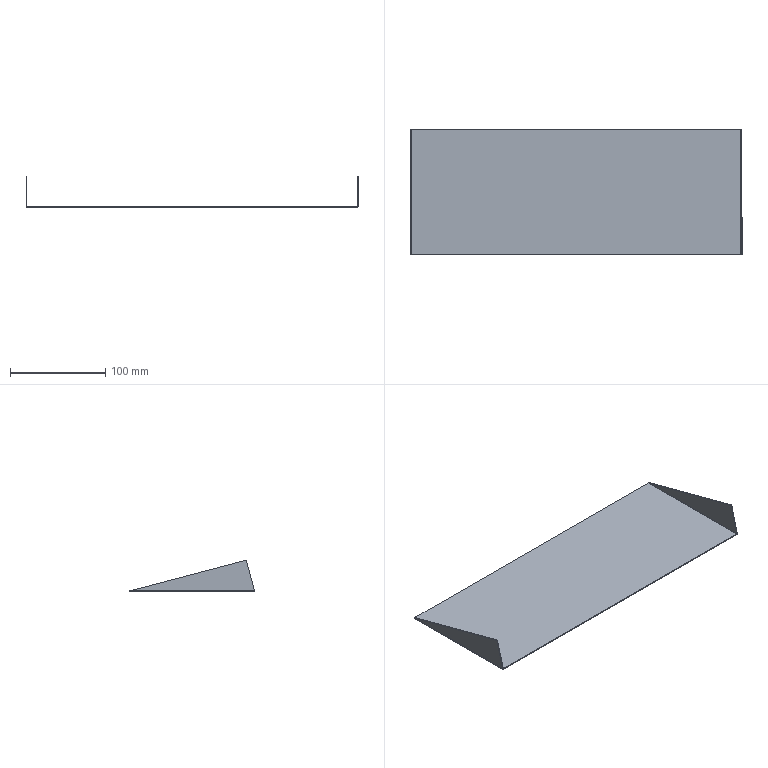Part | SolidWorks | features EdgeFlange 1, FlatPattern 1, MirrorPattern 1, SMBaseFlange 1, SheetMetal 1 | 1 solid | 20 faces | box 349.001 x 131.5 x 33.5 mm | volume 50088 mm3 | plane 12 | spline 4 | cylinder 4 | commonest cylinder face diameters 0.4 x2 2.4 x2
STEP:
#1=CARTESIAN_POINT('',(173.3,65.75,-1.));
#2=VERTEX_POINT('',#1);
#3=CARTESIAN_POINT('',(173.3,-65.75,-1.));
#4=VERTEX_POINT('',#3);
#5=CARTESIAN_POINT('',(173.3,65.75,-1.));
#6=DIRECTION('',(0.,-1.,0.));
#7=VECTOR('',#6,1000.);
#8=LINE('',#5,#7);
#9=EDGE_CURVE('',#2,#4,#8,.T.);
#10=ORIENTED_EDGE('',*,*,#9,.T.);
#11=CARTESIAN_POINT('',(-173.3,-65.75,-1.));
#12=VERTEX_POINT('',#11);
#13=CARTESIAN_POINT('',(-174.5,-65.75,-1.));
#14=DIRECTION('',(1.,0.,0.));
#15=VECTOR('',#14,1000.);
#16=LINE('',#13,#15);
#17=EDGE_CURVE('',#12,#4,#16,.T.);
#18=ORIENTED_EDGE('',*,*,#17,.F.);
#19=CARTESIAN_POINT('',(-173.3,65.75,-1.));
#20=VERTEX_POINT('',#19);
#21=CARTESIAN_POINT('',(-173.3,-65.75,-1.));
#22=DIRECTION('',(0.,1.,0.));
#23=VECTOR('',#22,1000.);
#24=LINE('',#21,#23);
#25=EDGE_CURVE('',#12,#20,#24,.T.);
#26=ORIENTED_EDGE('',*,*,#25,.T.);
#27=CARTESIAN_POINT('',(-174.5,65.75,-1.));
#28=DIRECTION('',(-1.,0.,0.));
#29=VECTOR('',#28,1000.);
#30=LINE('',#27,#29);
#31=EDGE_CURVE('',#2,#20,#30,.T.);
#32=ORIENTED_EDGE('',*,*,#31,.F.);
#33=EDGE_LOOP('',(#10,#18,#26,#32));
#34=FACE_OUTER_BOUND('',#33,.T.);
#35=CARTESIAN_POINT('',(0.,0.,-1.));
#36=DIRECTION('',(0.,0.,1.));
#37=DIRECTION('',(1.,0.,0.));
#38=AXIS2_PLACEMENT_3D('',#35,#36,#37);
#39=PLANE('',#38);
#40=ADVANCED_FACE('',(#34),#39,.F.);
#41=CARTESIAN_POINT('',(-173.3,-65.75,0.));
#42=VERTEX_POINT('',#41);
#43=CARTESIAN_POINT('',(173.3,-65.75,0.));
#44=VERTEX_POINT('',#43);
#45=CARTESIAN_POINT('',(-174.5,-65.75,0.));
#46=DIRECTION('',(1.,0.,0.));
#47=VECTOR('',#46,1000.);
#48=LINE('',#45,#47);
#49=EDGE_CURVE('',#42,#44,#48,.T.);
#50=ORIENTED_EDGE('',*,*,#49,.T.);
#51=CARTESIAN_POINT('',(173.3,65.75,0.));
#52=VERTEX_POINT('',#51);
#53=CARTESIAN_POINT('',(173.3,65.75,0.));
#54=DIRECTION('',(0.,-1.,0.));
#55=VECTOR('',#54,1000.);
#56=LINE('',#53,#55);
#57=EDGE_CURVE('',#52,#44,#56,.T.);
#58=ORIENTED_EDGE('',*,*,#57,.F.);
#59=CARTESIAN_POINT('',(-173.3,65.75,0.));
#60=VERTEX_POINT('',#59);
#61=CARTESIAN_POINT('',(-174.5,65.75,0.));
#62=DIRECTION('',(-1.,0.,0.));
#63=VECTOR('',#62,1000.);
#64=LINE('',#61,#63);
#65=EDGE_CURVE('',#52,#60,#64,.T.);
#66=ORIENTED_EDGE('',*,*,#65,.T.);
#67=CARTESIAN_POINT('',(-173.3,-65.75,0.));
#68=DIRECTION('',(0.,1.,0.));
#69=VECTOR('',#68,1000.);
#70=LINE('',#67,#69);
#71=EDGE_CURVE('',#42,#60,#70,.T.);
#72=ORIENTED_EDGE('',*,*,#71,.F.);
#73=EDGE_LOOP('',(#50,#58,#66,#72));
#74=FACE_OUTER_BOUND('',#73,.T.);
#75=CARTESIAN_POINT('',(0.,0.,0.));
#76=DIRECTION('',(0.,0.,1.));
#77=DIRECTION('',(1.,0.,0.));
#78=AXIS2_PLACEMENT_3D('',#75,#76,#77);
#79=PLANE('',#78);
#80=ADVANCED_FACE('',(#74),#79,.T.);
#81=ORIENTED_EDGE('',*,*,#65,.F.);
#82=CARTESIAN_POINT('',(173.3,65.75,0.));
#83=DIRECTION('',(0.,0.,-1.));
#84=VECTOR('',#83,1000.);
#85=LINE('',#82,#84);
#86=EDGE_CURVE('',#52,#2,#85,.T.);
#87=ORIENTED_EDGE('',*,*,#86,.T.);
#88=ORIENTED_EDGE('',*,*,#31,.T.);
#89=CARTESIAN_POINT('',(-173.3,65.75,0.));
#90=DIRECTION('',(0.,0.,-1.));
#91=VECTOR('',#90,1000.);
#92=LINE('',#89,#91);
#93=EDGE_CURVE('',#60,#20,#92,.T.);
#94=ORIENTED_EDGE('',*,*,#93,.F.);
#95=EDGE_LOOP('',(#81,#87,#88,#94));
#96=FACE_OUTER_BOUND('',#95,.T.);
#97=CARTESIAN_POINT('',(-174.5,65.75,-1.));
#98=DIRECTION('',(0.,1.,0.));
#99=DIRECTION('',(0.,0.,1.));
#100=AXIS2_PLACEMENT_3D('',#97,#98,#99);
#101=PLANE('',#100);
#102=ADVANCED_FACE('',(#96),#101,.T.);
#103=CARTESIAN_POINT('',(173.3,-65.75,0.));
#104=DIRECTION('',(0.,0.,-1.));
#105=VECTOR('',#104,1000.);
#106=LINE('',#103,#105);
#107=EDGE_CURVE('',#44,#4,#106,.T.);
#108=ORIENTED_EDGE('',*,*,#107,.F.);
#109=ORIENTED_EDGE('',*,*,#49,.F.);
#110=CARTESIAN_POINT('',(-173.3,-65.75,0.));
#111=DIRECTION('',(0.,0.,-1.));
#112=VECTOR('',#111,1000.);
#113=LINE('',#110,#112);
#114=EDGE_CURVE('',#42,#12,#113,.T.);
#115=ORIENTED_EDGE('',*,*,#114,.T.);
#116=ORIENTED_EDGE('',*,*,#17,.T.);
#117=EDGE_LOOP('',(#108,#109,#115,#116));
#118=FACE_OUTER_BOUND('',#117,.T.);
#119=CARTESIAN_POINT('',(-174.5,-65.75,-1.));
#120=DIRECTION('',(0.,-1.,0.));
#121=DIRECTION('',(0.,0.,-1.));
#122=AXIS2_PLACEMENT_3D('',#119,#120,#121);
#123=PLANE('',#122);
#124=ADVANCED_FACE('',(#118),#123,.T.);
#125=CARTESIAN_POINT('',(-173.5,64.994,0.2));
#126=VERTEX_POINT('',#125);
#127=CARTESIAN_POINT('',(-174.5,64.994,0.2));
#128=VERTEX_POINT('',#127);
#129=CARTESIAN_POINT('',(-174.5,64.994,0.2));
#130=DIRECTION('',(-1.,0.,0.));
#131=VECTOR('',#130,1000.);
#132=LINE('',#129,#131);
#133=EDGE_CURVE('',#126,#128,#132,.T.);
#134=ORIENTED_EDGE('',*,*,#133,.F.);
#135=CARTESIAN_POINT('',(-173.3,65.75,0.));
#136=CARTESIAN_POINT('',(-173.352,65.624,0.));
#137=CARTESIAN_POINT('',(-173.404,65.498,0.02155));
#138=CARTESIAN_POINT('',(-173.478,65.246,0.0956));
#139=CARTESIAN_POINT('',(-173.5,65.12,0.1476));
#140=CARTESIAN_POINT('',(-173.5,64.994,0.2));
#141=B_SPLINE_CURVE_WITH_KNOTS('',3,(#135,#136,#137,#138,#139,#140),.UNSPECIFIED.,.F.,.F.,(4,2,4),(0.,0.5,1.),.UNSPECIFIED.);
#142=EDGE_CURVE('',#60,#126,#141,.T.);
#143=ORIENTED_EDGE('',*,*,#142,.F.);
#144=ORIENTED_EDGE('',*,*,#93,.T.);
#145=CARTESIAN_POINT('',(-173.3,65.75,-1.));
#146=CARTESIAN_POINT('',(-173.459,65.686,-1.));
#147=CARTESIAN_POINT('',(-173.612,65.625,-0.9695));
#148=CARTESIAN_POINT('',(-173.905,65.498,-0.8485));
#149=CARTESIAN_POINT('',(-174.036,65.436,-0.7607));
#150=CARTESIAN_POINT('',(-174.26,65.309,-0.5373));
#151=CARTESIAN_POINT('',(-174.348,65.246,-0.4052));
#152=CARTESIAN_POINT('',(-174.469,65.12,-0.1142));
#153=CARTESIAN_POINT('',(-174.5,65.057,0.04141));
#154=CARTESIAN_POINT('',(-174.5,64.994,0.2));
#155=B_SPLINE_CURVE_WITH_KNOTS('',3,(#145,#146,#147,#148,#149,#150,#151,#152,#153,#154),.UNSPECIFIED.,.F.,.F.,(4,2,2,2,4),(0.,0.0005039,0.001008,0.001512,0.002016),.UNSPECIFIED.);
#156=EDGE_CURVE('',#20,#128,#155,.T.);
#157=ORIENTED_EDGE('',*,*,#156,.T.);
#158=EDGE_LOOP('',(#134,#143,#144,#157));
#159=FACE_OUTER_BOUND('',#158,.T.);
#160=CARTESIAN_POINT('',(-173.3,65.75,-1.01));
#161=CARTESIAN_POINT('',(-173.458,65.687,-1.01));
#162=CARTESIAN_POINT('',(-173.617,65.624,-0.9785));
#163=CARTESIAN_POINT('',(-173.909,65.498,-0.8573));
#164=CARTESIAN_POINT('',(-174.044,65.435,-0.7676));
#165=CARTESIAN_POINT('',(-174.268,65.309,-0.5436));
#166=CARTESIAN_POINT('',(-174.357,65.246,-0.4094));
#167=CARTESIAN_POINT('',(-174.479,65.12,-0.1167));
#168=CARTESIAN_POINT('',(-174.51,65.057,0.04159));
#169=CARTESIAN_POINT('',(-174.51,64.994,0.2));
#170=CARTESIAN_POINT('',(-173.3,65.75,-1.));
#171=CARTESIAN_POINT('',(-173.457,65.687,-1.));
#172=CARTESIAN_POINT('',(-173.614,65.624,-0.9688));
#173=CARTESIAN_POINT('',(-173.904,65.498,-0.8485));
#174=CARTESIAN_POINT('',(-174.037,65.435,-0.7596));
#175=CARTESIAN_POINT('',(-174.26,65.309,-0.5375));
#176=CARTESIAN_POINT('',(-174.349,65.246,-0.4043));
#177=CARTESIAN_POINT('',(-174.469,65.12,-0.1141));
#178=CARTESIAN_POINT('',(-174.5,65.057,0.0429));
#179=CARTESIAN_POINT('',(-174.5,64.994,0.2));
#180=CARTESIAN_POINT('',(-173.3,65.75,0.));
#181=CARTESIAN_POINT('',(-173.326,65.687,0.));
#182=CARTESIAN_POINT('',(-173.352,65.624,0.005205));
#183=CARTESIAN_POINT('',(-173.401,65.498,0.02524));
#184=CARTESIAN_POINT('',(-173.423,65.435,0.04007));
#185=CARTESIAN_POINT('',(-173.46,65.309,0.07709));
#186=CARTESIAN_POINT('',(-173.475,65.246,0.09928));
#187=CARTESIAN_POINT('',(-173.495,65.12,0.1477));
#188=CARTESIAN_POINT('',(-173.5,65.057,0.1738));
#189=CARTESIAN_POINT('',(-173.5,64.994,0.2));
#190=B_SPLINE_SURFACE_WITH_KNOTS('',1,3,((#160,#161,#162,#163,#164,#165,#166,#167,#168,#169),(#170,#171,#172,#173,#174,#175,#176,#177,#178,#179),(#180,#181,#182,#183,#184,#185,#186,#187,#188,#189)),.UNSPECIFIED.,.F.,.F.,.F.,(2,1,2),(4,2,2,2,4),(-0.01,0.,1.),(0.,0.25,0.5,0.75,1.),.UNSPECIFIED.);
#191=ADVANCED_FACE('',(#159),#190,.F.);
#192=CARTESIAN_POINT('',(-173.5,-65.697,0.2));
#193=VERTEX_POINT('',#192);
#194=CARTESIAN_POINT('',(-173.5,-65.697,0.2));
#195=CARTESIAN_POINT('',(-173.5,-65.706,0.1476));
#196=CARTESIAN_POINT('',(-173.478,-65.715,0.0956));
#197=CARTESIAN_POINT('',(-173.404,-65.732,0.02155));
#198=CARTESIAN_POINT('',(-173.352,-65.741,0.));
#199=CARTESIAN_POINT('',(-173.3,-65.75,0.));
#200=B_SPLINE_CURVE_WITH_KNOTS('',3,(#194,#195,#196,#197,#198,#199),.UNSPECIFIED.,.F.,.F.,(4,2,4),(0.,0.5,1.),.UNSPECIFIED.);
#201=EDGE_CURVE('',#193,#42,#200,.T.);
#202=ORIENTED_EDGE('',*,*,#201,.F.);
#203=CARTESIAN_POINT('',(-174.5,-65.697,0.2));
#204=VERTEX_POINT('',#203);
#205=CARTESIAN_POINT('',(-173.5,-65.697,0.2));
#206=DIRECTION('',(-1.,0.,0.));
#207=VECTOR('',#206,1000.);
#208=LINE('',#205,#207);
#209=EDGE_CURVE('',#193,#204,#208,.T.);
#210=ORIENTED_EDGE('',*,*,#209,.T.);
#211=CARTESIAN_POINT('',(-174.5,-65.697,0.2));
#212=CARTESIAN_POINT('',(-174.5,-65.702,0.04292));
#213=CARTESIAN_POINT('',(-174.469,-65.706,-0.1141));
#214=CARTESIAN_POINT('',(-174.349,-65.715,-0.4043));
#215=CARTESIAN_POINT('',(-174.26,-65.719,-0.5375));
#216=CARTESIAN_POINT('',(-174.037,-65.728,-0.7596));
#217=CARTESIAN_POINT('',(-173.904,-65.732,-0.8485));
#218=CARTESIAN_POINT('',(-173.614,-65.741,-0.9688));
#219=CARTESIAN_POINT('',(-173.457,-65.746,-1.));
#220=CARTESIAN_POINT('',(-173.3,-65.75,-1.));
#221=B_SPLINE_CURVE_WITH_KNOTS('',3,(#211,#212,#213,#214,#215,#216,#217,#218,#219,#220),.UNSPECIFIED.,.F.,.F.,(4,2,2,2,4),(0.,0.25,0.5,0.75,1.),.UNSPECIFIED.);
#222=EDGE_CURVE('',#204,#12,#221,.T.);
#223=ORIENTED_EDGE('',*,*,#222,.T.);
#224=ORIENTED_EDGE('',*,*,#114,.F.);
#225=EDGE_LOOP('',(#202,#210,#223,#224));
#226=FACE_OUTER_BOUND('',#225,.T.);
#227=CARTESIAN_POINT('',(-174.51,-65.697,0.2));
#228=CARTESIAN_POINT('',(-174.51,-65.702,0.04158));
#229=CARTESIAN_POINT('',(-174.479,-65.706,-0.1167));
#230=CARTESIAN_POINT('',(-174.357,-65.715,-0.4094));
#231=CARTESIAN_POINT('',(-174.268,-65.719,-0.5436));
#232=CARTESIAN_POINT('',(-174.044,-65.728,-0.7676));
#233=CARTESIAN_POINT('',(-173.909,-65.732,-0.8573));
#234=CARTESIAN_POINT('',(-173.617,-65.741,-0.9785));
#235=CARTESIAN_POINT('',(-173.458,-65.746,-1.01));
#236=CARTESIAN_POINT('',(-173.3,-65.75,-1.01));
#237=CARTESIAN_POINT('',(-174.5,-65.697,0.2));
#238=CARTESIAN_POINT('',(-174.5,-65.702,0.04289));
#239=CARTESIAN_POINT('',(-174.469,-65.706,-0.1141));
#240=CARTESIAN_POINT('',(-174.349,-65.715,-0.4043));
#241=CARTESIAN_POINT('',(-174.26,-65.719,-0.5375));
#242=CARTESIAN_POINT('',(-174.037,-65.728,-0.7596));
#243=CARTESIAN_POINT('',(-173.904,-65.732,-0.8485));
#244=CARTESIAN_POINT('',(-173.614,-65.741,-0.9688));
#245=CARTESIAN_POINT('',(-173.457,-65.746,-1.));
#246=CARTESIAN_POINT('',(-173.3,-65.75,-1.));
#247=CARTESIAN_POINT('',(-173.5,-65.697,0.2));
#248=CARTESIAN_POINT('',(-173.5,-65.702,0.1738));
#249=CARTESIAN_POINT('',(-173.495,-65.706,0.1477));
#250=CARTESIAN_POINT('',(-173.475,-65.715,0.09928));
#251=CARTESIAN_POINT('',(-173.46,-65.719,0.07709));
#252=CARTESIAN_POINT('',(-173.423,-65.728,0.04007));
#253=CARTESIAN_POINT('',(-173.401,-65.732,0.02524));
#254=CARTESIAN_POINT('',(-173.352,-65.741,0.005205));
#255=CARTESIAN_POINT('',(-173.326,-65.746,0.));
#256=CARTESIAN_POINT('',(-173.3,-65.75,0.));
#257=CARTESIAN_POINT('',(-173.49,-65.697,0.2));
#258=CARTESIAN_POINT('',(-173.49,-65.702,0.1751));
#259=CARTESIAN_POINT('',(-173.485,-65.706,0.1503));
#260=CARTESIAN_POINT('',(-173.466,-65.715,0.1044));
#261=CARTESIAN_POINT('',(-173.452,-65.719,0.0833));
#262=CARTESIAN_POINT('',(-173.417,-65.728,0.04814));
#263=CARTESIAN_POINT('',(-173.396,-65.732,0.03407));
#264=CARTESIAN_POINT('',(-173.35,-65.741,0.01504));
#265=CARTESIAN_POINT('',(-173.325,-65.746,0.0101));
#266=CARTESIAN_POINT('',(-173.3,-65.75,0.0101));
#267=B_SPLINE_SURFACE_WITH_KNOTS('',1,3,((#227,#228,#229,#230,#231,#232,#233,#234,#235,#236),(#237,#238,#239,#240,#241,#242,#243,#244,#245,#246),(#247,#248,#249,#250,#251,#252,#253,#254,#255,#256),(#257,#258,#259,#260,#261,#262,#263,#264,#265,#266)),.UNSPECIFIED.,.F.,.F.,.F.,(2,1,1,2),(4,2,2,2,4),(-0.01,0.,1.,1.01),(0.,0.25,0.5,0.75,1.),.UNSPECIFIED.);
#268=ADVANCED_FACE('',(#226),#267,.F.);
#269=ORIENTED_EDGE('',*,*,#25,.F.);
#270=ORIENTED_EDGE('',*,*,#222,.F.);
#271=CARTESIAN_POINT('',(-174.5,64.994,0.2));
#272=DIRECTION('',(0.,1.,0.));
#273=VECTOR('',#272,1000.);
#274=LINE('',#271,#273);
#275=EDGE_CURVE('',#204,#128,#274,.T.);
#276=ORIENTED_EDGE('',*,*,#275,.T.);
#277=ORIENTED_EDGE('',*,*,#156,.F.);
#278=EDGE_LOOP('',(#269,#270,#276,#277));
#279=FACE_OUTER_BOUND('',#278,.T.);
#280=CARTESIAN_POINT('',(-173.3,-65.75,0.2));
#281=DIRECTION('',(0.,-1.,0.));
#282=DIRECTION('',(-1.,0.,0.));
#283=AXIS2_PLACEMENT_3D('',#280,#281,#282);
#284=CYLINDRICAL_SURFACE('',#283,1.2);
#285=ADVANCED_FACE('',(#279),#284,.T.);
#286=ORIENTED_EDGE('',*,*,#71,.T.);
#287=ORIENTED_EDGE('',*,*,#142,.T.);
#288=CARTESIAN_POINT('',(-173.5,64.994,0.2));
#289=DIRECTION('',(0.,-1.,0.));
#290=VECTOR('',#289,1000.);
#291=LINE('',#288,#290);
#292=EDGE_CURVE('',#126,#193,#291,.T.);
#293=ORIENTED_EDGE('',*,*,#292,.T.);
#294=ORIENTED_EDGE('',*,*,#201,.T.);
#295=EDGE_LOOP('',(#286,#287,#293,#294));
#296=FACE_OUTER_BOUND('',#295,.T.);
#297=CARTESIAN_POINT('',(-173.3,-65.75,0.2));
#298=DIRECTION('',(0.,-1.,0.));
#299=DIRECTION('',(-1.,0.,0.));
#300=AXIS2_PLACEMENT_3D('',#297,#298,#299);
#301=CYLINDRICAL_SURFACE('',#300,0.2);
#302=ADVANCED_FACE('',(#296),#301,.F.);
#303=ORIENTED_EDGE('',*,*,#133,.T.);
#304=CARTESIAN_POINT('',(-174.5,-57.156,32.5));
#305=VERTEX_POINT('',#304);
#306=CARTESIAN_POINT('',(-174.5,4.297,16.25));
#307=DIRECTION('',(0.,0.9668,-0.2556));
#308=VECTOR('',#307,1000.);
#309=LINE('',#306,#308);
#310=EDGE_CURVE('',#305,#128,#309,.T.);
#311=ORIENTED_EDGE('',*,*,#310,.F.);
#312=CARTESIAN_POINT('',(-173.5,-57.156,32.5));
#313=VERTEX_POINT('',#312);
#314=CARTESIAN_POINT('',(-174.5,-57.156,32.5));
#315=DIRECTION('',(1.,0.,0.));
#316=VECTOR('',#315,1000.);
#317=LINE('',#314,#316);
#318=EDGE_CURVE('',#305,#313,#317,.T.);
#319=ORIENTED_EDGE('',*,*,#318,.T.);
#320=CARTESIAN_POINT('',(-173.5,-57.156,32.5));
#321=DIRECTION('',(0.,0.9668,-0.2556));
#322=VECTOR('',#321,1000.);
#323=LINE('',#320,#322);
#324=EDGE_CURVE('',#313,#126,#323,.T.);
#325=ORIENTED_EDGE('',*,*,#324,.T.);
#326=EDGE_LOOP('',(#303,#311,#319,#325));
#327=FACE_OUTER_BOUND('',#326,.T.);
#328=CARTESIAN_POINT('',(-174.5,-57.156,32.5));
#329=DIRECTION('',(0.,-0.2556,-0.9668));
#330=DIRECTION('',(0.,0.9668,-0.2556));
#331=AXIS2_PLACEMENT_3D('',#328,#329,#330);
#332=PLANE('',#331);
#333=ADVANCED_FACE('',(#327),#332,.F.);
#334=ORIENTED_EDGE('',*,*,#209,.F.);
#335=CARTESIAN_POINT('',(-173.5,-65.75,0.));
#336=DIRECTION('',(0.,0.2556,0.9668));
#337=VECTOR('',#336,1000.);
#338=LINE('',#335,#337);
#339=EDGE_CURVE('',#193,#313,#338,.T.);
#340=ORIENTED_EDGE('',*,*,#339,.T.);
#341=ORIENTED_EDGE('',*,*,#318,.F.);
#342=CARTESIAN_POINT('',(-174.5,-61.453,16.25));
#343=DIRECTION('',(0.,0.2556,0.9668));
#344=VECTOR('',#343,1000.);
#345=LINE('',#342,#344);
#346=EDGE_CURVE('',#204,#305,#345,.T.);
#347=ORIENTED_EDGE('',*,*,#346,.F.);
#348=EDGE_LOOP('',(#334,#340,#341,#347));
#349=FACE_OUTER_BOUND('',#348,.T.);
#350=CARTESIAN_POINT('',(-174.5,-65.75,0.));
#351=DIRECTION('',(0.,0.9668,-0.2556));
#352=DIRECTION('',(0.,0.2556,0.9668));
#353=AXIS2_PLACEMENT_3D('',#350,#351,#352);
#354=PLANE('',#353);
#355=ADVANCED_FACE('',(#349),#354,.F.);
#356=ORIENTED_EDGE('',*,*,#275,.F.);
#357=ORIENTED_EDGE('',*,*,#346,.T.);
#358=ORIENTED_EDGE('',*,*,#310,.T.);
#359=EDGE_LOOP('',(#356,#357,#358));
#360=FACE_OUTER_BOUND('',#359,.T.);
#361=CARTESIAN_POINT('',(-174.5,0.,0.));
#362=DIRECTION('',(1.,0.,0.));
#363=DIRECTION('',(0.,0.,-1.));
#364=AXIS2_PLACEMENT_3D('',#361,#362,#363);
#365=PLANE('',#364);
#366=ADVANCED_FACE('',(#360),#365,.F.);
#367=ORIENTED_EDGE('',*,*,#339,.F.);
#368=ORIENTED_EDGE('',*,*,#292,.F.);
#369=ORIENTED_EDGE('',*,*,#324,.F.);
#370=EDGE_LOOP('',(#367,#368,#369));
#371=FACE_OUTER_BOUND('',#370,.T.);
#372=CARTESIAN_POINT('',(-173.5,0.,0.));
#373=DIRECTION('',(1.,0.,0.));
#374=DIRECTION('',(0.,0.,-1.));
#375=AXIS2_PLACEMENT_3D('',#372,#373,#374);
#376=PLANE('',#375);
#377=ADVANCED_FACE('',(#371),#376,.T.);
#378=CARTESIAN_POINT('',(173.5,-65.697,0.2));
#379=VERTEX_POINT('',#378);
#380=CARTESIAN_POINT('',(174.5,-65.697,0.2));
#381=VERTEX_POINT('',#380);
#382=CARTESIAN_POINT('',(174.5,-65.697,0.2));
#383=DIRECTION('',(1.,0.,0.));
#384=VECTOR('',#383,1000.);
#385=LINE('',#382,#384);
#386=EDGE_CURVE('',#379,#381,#385,.T.);
#387=ORIENTED_EDGE('',*,*,#386,.F.);
#388=CARTESIAN_POINT('',(173.3,-65.75,0.));
#389=CARTESIAN_POINT('',(173.352,-65.741,0.));
#390=CARTESIAN_POINT('',(173.404,-65.732,0.02155));
#391=CARTESIAN_POINT('',(173.478,-65.715,0.0956));
#392=CARTESIAN_POINT('',(173.5,-65.706,0.1476));
#393=CARTESIAN_POINT('',(173.5,-65.697,0.2));
#394=B_SPLINE_CURVE_WITH_KNOTS('',3,(#388,#389,#390,#391,#392,#393),.UNSPECIFIED.,.F.,.F.,(4,2,4),(0.,0.5,1.),.UNSPECIFIED.);
#395=EDGE_CURVE('',#44,#379,#394,.T.);
#396=ORIENTED_EDGE('',*,*,#395,.F.);
#397=ORIENTED_EDGE('',*,*,#107,.T.);
#398=CARTESIAN_POINT('',(173.3,-65.75,-1.));
#399=CARTESIAN_POINT('',(173.457,-65.746,-1.));
#400=CARTESIAN_POINT('',(173.614,-65.741,-0.9688));
#401=CARTESIAN_POINT('',(173.904,-65.732,-0.8485));
#402=CARTESIAN_POINT('',(174.037,-65.728,-0.7596));
#403=CARTESIAN_POINT('',(174.26,-65.719,-0.5375));
#404=CARTESIAN_POINT('',(174.349,-65.715,-0.4043));
#405=CARTESIAN_POINT('',(174.469,-65.706,-0.1141));
#406=CARTESIAN_POINT('',(174.5,-65.702,0.04292));
#407=CARTESIAN_POINT('',(174.5,-65.697,0.2));
#408=B_SPLINE_CURVE_WITH_KNOTS('',3,(#398,#399,#400,#401,#402,#403,#404,#405,#406,#407),.UNSPECIFIED.,.F.,.F.,(4,2,2,2,4),(0.,0.25,0.5,0.75,1.),.UNSPECIFIED.);
#409=EDGE_CURVE('',#4,#381,#408,.T.);
#410=ORIENTED_EDGE('',*,*,#409,.T.);
#411=EDGE_LOOP('',(#387,#396,#397,#410));
#412=FACE_OUTER_BOUND('',#411,.T.);
#413=CARTESIAN_POINT('',(173.3,-65.75,-1.01));
#414=CARTESIAN_POINT('',(173.458,-65.746,-1.01));
#415=CARTESIAN_POINT('',(173.617,-65.741,-0.9785));
#416=CARTESIAN_POINT('',(173.909,-65.732,-0.8573));
#417=CARTESIAN_POINT('',(174.044,-65.728,-0.7676));
#418=CARTESIAN_POINT('',(174.268,-65.719,-0.5436));
#419=CARTESIAN_POINT('',(174.357,-65.715,-0.4094));
#420=CARTESIAN_POINT('',(174.479,-65.706,-0.1167));
#421=CARTESIAN_POINT('',(174.51,-65.702,0.04158));
#422=CARTESIAN_POINT('',(174.51,-65.697,0.2));
#423=CARTESIAN_POINT('',(173.3,-65.75,-1.));
#424=CARTESIAN_POINT('',(173.457,-65.746,-1.));
#425=CARTESIAN_POINT('',(173.614,-65.741,-0.9688));
#426=CARTESIAN_POINT('',(173.904,-65.732,-0.8485));
#427=CARTESIAN_POINT('',(174.037,-65.728,-0.7596));
#428=CARTESIAN_POINT('',(174.26,-65.719,-0.5375));
#429=CARTESIAN_POINT('',(174.349,-65.715,-0.4043));
#430=CARTESIAN_POINT('',(174.469,-65.706,-0.1141));
#431=CARTESIAN_POINT('',(174.5,-65.702,0.04289));
#432=CARTESIAN_POINT('',(174.5,-65.697,0.2));
#433=CARTESIAN_POINT('',(173.3,-65.75,0.));
#434=CARTESIAN_POINT('',(173.326,-65.746,0.));
#435=CARTESIAN_POINT('',(173.352,-65.741,0.005205));
#436=CARTESIAN_POINT('',(173.401,-65.732,0.02524));
#437=CARTESIAN_POINT('',(173.423,-65.728,0.04007));
#438=CARTESIAN_POINT('',(173.46,-65.719,0.07709));
#439=CARTESIAN_POINT('',(173.475,-65.715,0.09928));
#440=CARTESIAN_POINT('',(173.495,-65.706,0.1477));
#441=CARTESIAN_POINT('',(173.5,-65.702,0.1738));
#442=CARTESIAN_POINT('',(173.5,-65.697,0.2));
#443=CARTESIAN_POINT('',(173.3,-65.75,0.0101));
#444=CARTESIAN_POINT('',(173.325,-65.746,0.0101));
#445=CARTESIAN_POINT('',(173.35,-65.741,0.01504));
#446=CARTESIAN_POINT('',(173.396,-65.732,0.03407));
#447=CARTESIAN_POINT('',(173.417,-65.728,0.04814));
#448=CARTESIAN_POINT('',(173.452,-65.719,0.0833));
#449=CARTESIAN_POINT('',(173.466,-65.715,0.1044));
#450=CARTESIAN_POINT('',(173.485,-65.706,0.1503));
#451=CARTESIAN_POINT('',(173.49,-65.702,0.1751));
#452=CARTESIAN_POINT('',(173.49,-65.697,0.2));
#453=B_SPLINE_SURFACE_WITH_KNOTS('',1,3,((#413,#414,#415,#416,#417,#418,#419,#420,#421,#422),(#423,#424,#425,#426,#427,#428,#429,#430,#431,#432),(#433,#434,#435,#436,#437,#438,#439,#440,#441,#442),(#443,#444,#445,#446,#447,#448,#449,#450,#451,#452)),.UNSPECIFIED.,.F.,.F.,.F.,(2,1,1,2),(4,2,2,2,4),(-0.01,0.,1.,1.01),(0.,0.25,0.5,0.75,1.),.UNSPECIFIED.);
#454=ADVANCED_FACE('',(#412),#453,.F.);
#455=CARTESIAN_POINT('',(173.5,64.994,0.2));
#456=VERTEX_POINT('',#455);
#457=CARTESIAN_POINT('',(173.5,64.994,0.2));
#458=CARTESIAN_POINT('',(173.5,65.12,0.1476));
#459=CARTESIAN_POINT('',(173.478,65.246,0.0956));
#460=CARTESIAN_POINT('',(173.404,65.498,0.02155));
#461=CARTESIAN_POINT('',(173.352,65.624,0.));
#462=CARTESIAN_POINT('',(173.3,65.75,0.));
#463=B_SPLINE_CURVE_WITH_KNOTS('',3,(#457,#458,#459,#460,#461,#462),.UNSPECIFIED.,.F.,.F.,(4,2,4),(0.,0.5,1.),.UNSPECIFIED.);
#464=EDGE_CURVE('',#456,#52,#463,.T.);
#465=ORIENTED_EDGE('',*,*,#464,.F.);
#466=CARTESIAN_POINT('',(174.5,64.994,0.2));
#467=VERTEX_POINT('',#466);
#468=CARTESIAN_POINT('',(173.5,64.994,0.2));
#469=DIRECTION('',(1.,0.,0.));
#470=VECTOR('',#469,1000.);
#471=LINE('',#468,#470);
#472=EDGE_CURVE('',#456,#467,#471,.T.);
#473=ORIENTED_EDGE('',*,*,#472,.T.);
#474=CARTESIAN_POINT('',(174.5,64.994,0.2));
#475=CARTESIAN_POINT('',(174.5,65.057,0.04141));
#476=CARTESIAN_POINT('',(174.47,65.119,-0.1119));
#477=CARTESIAN_POINT('',(174.349,65.246,-0.4047));
#478=CARTESIAN_POINT('',(174.261,65.308,-0.5362));
#479=CARTESIAN_POINT('',(174.037,65.435,-0.7599));
#480=CARTESIAN_POINT('',(173.905,65.498,-0.8481));
#481=CARTESIAN_POINT('',(173.614,65.624,-0.9688));
#482=CARTESIAN_POINT('',(173.459,65.686,-1.));
#483=CARTESIAN_POINT('',(173.3,65.75,-1.));
#484=B_SPLINE_CURVE_WITH_KNOTS('',3,(#474,#475,#476,#477,#478,#479,#480,#481,#482,#483),.UNSPECIFIED.,.F.,.F.,(4,2,2,2,4),(0.,0.0005039,0.001008,0.001512,0.002016),.UNSPECIFIED.);
#485=EDGE_CURVE('',#467,#2,#484,.T.);
#486=ORIENTED_EDGE('',*,*,#485,.T.);
#487=ORIENTED_EDGE('',*,*,#86,.F.);
#488=EDGE_LOOP('',(#465,#473,#486,#487));
#489=FACE_OUTER_BOUND('',#488,.T.);
#490=CARTESIAN_POINT('',(174.51,64.994,0.2));
#491=CARTESIAN_POINT('',(174.51,65.057,0.04159));
#492=CARTESIAN_POINT('',(174.479,65.12,-0.1167));
#493=CARTESIAN_POINT('',(174.357,65.246,-0.4094));
#494=CARTESIAN_POINT('',(174.268,65.309,-0.5436));
#495=CARTESIAN_POINT('',(174.044,65.435,-0.7676));
#496=CARTESIAN_POINT('',(173.909,65.498,-0.8573));
#497=CARTESIAN_POINT('',(173.617,65.624,-0.9785));
#498=CARTESIAN_POINT('',(173.458,65.687,-1.01));
#499=CARTESIAN_POINT('',(173.3,65.75,-1.01));
#500=CARTESIAN_POINT('',(174.5,64.994,0.2));
#501=CARTESIAN_POINT('',(174.5,65.057,0.0429));
#502=CARTESIAN_POINT('',(174.469,65.12,-0.1141));
#503=CARTESIAN_POINT('',(174.349,65.246,-0.4043));
#504=CARTESIAN_POINT('',(174.26,65.309,-0.5375));
#505=CARTESIAN_POINT('',(174.037,65.435,-0.7596));
#506=CARTESIAN_POINT('',(173.904,65.498,-0.8485));
#507=CARTESIAN_POINT('',(173.614,65.624,-0.9688));
#508=CARTESIAN_POINT('',(173.457,65.687,-1.));
#509=CARTESIAN_POINT('',(173.3,65.75,-1.));
#510=CARTESIAN_POINT('',(173.5,64.994,0.2));
#511=CARTESIAN_POINT('',(173.5,65.057,0.1738));
#512=CARTESIAN_POINT('',(173.495,65.12,0.1477));
#513=CARTESIAN_POINT('',(173.475,65.246,0.09928));
#514=CARTESIAN_POINT('',(173.46,65.309,0.07709));
#515=CARTESIAN_POINT('',(173.423,65.435,0.04007));
#516=CARTESIAN_POINT('',(173.401,65.498,0.02524));
#517=CARTESIAN_POINT('',(173.352,65.624,0.005205));
#518=CARTESIAN_POINT('',(173.326,65.687,0.));
#519=CARTESIAN_POINT('',(173.3,65.75,0.));
#520=B_SPLINE_SURFACE_WITH_KNOTS('',1,3,((#490,#491,#492,#493,#494,#495,#496,#497,#498,#499),(#500,#501,#502,#503,#504,#505,#506,#507,#508,#509),(#510,#511,#512,#513,#514,#515,#516,#517,#518,#519)),.UNSPECIFIED.,.F.,.F.,.F.,(2,1,2),(4,2,2,2,4),(-0.01,0.,1.),(0.,0.25,0.5,0.75,1.),.UNSPECIFIED.);
#521=ADVANCED_FACE('',(#489),#520,.F.);
#522=ORIENTED_EDGE('',*,*,#9,.F.);
#523=ORIENTED_EDGE('',*,*,#485,.F.);
#524=CARTESIAN_POINT('',(174.5,-65.697,0.2));
#525=DIRECTION('',(0.,-1.,0.));
#526=VECTOR('',#525,1000.);
#527=LINE('',#524,#526);
#528=EDGE_CURVE('',#467,#381,#527,.T.);
#529=ORIENTED_EDGE('',*,*,#528,.T.);
#530=ORIENTED_EDGE('',*,*,#409,.F.);
#531=EDGE_LOOP('',(#522,#523,#529,#530));
#532=FACE_OUTER_BOUND('',#531,.T.);
#533=CARTESIAN_POINT('',(173.3,65.75,0.2));
#534=DIRECTION('',(0.,1.,0.));
#535=DIRECTION('',(1.,0.,0.));
#536=AXIS2_PLACEMENT_3D('',#533,#534,#535);
#537=CYLINDRICAL_SURFACE('',#536,1.2);
#538=ADVANCED_FACE('',(#532),#537,.T.);
#539=ORIENTED_EDGE('',*,*,#57,.T.);
#540=ORIENTED_EDGE('',*,*,#395,.T.);
#541=CARTESIAN_POINT('',(173.5,-65.697,0.2));
#542=DIRECTION('',(0.,1.,0.));
#543=VECTOR('',#542,1000.);
#544=LINE('',#541,#543);
#545=EDGE_CURVE('',#379,#456,#544,.T.);
#546=ORIENTED_EDGE('',*,*,#545,.T.);
#547=ORIENTED_EDGE('',*,*,#464,.T.);
#548=EDGE_LOOP('',(#539,#540,#546,#547));
#549=FACE_OUTER_BOUND('',#548,.T.);
#550=CARTESIAN_POINT('',(173.3,65.75,0.2));
#551=DIRECTION('',(0.,1.,0.));
#552=DIRECTION('',(1.,0.,0.));
#553=AXIS2_PLACEMENT_3D('',#550,#551,#552);
#554=CYLINDRICAL_SURFACE('',#553,0.2);
#555=ADVANCED_FACE('',(#549),#554,.F.);
#556=CARTESIAN_POINT('',(174.5,-57.156,32.5));
#557=VERTEX_POINT('',#556);
#558=CARTESIAN_POINT('',(174.5,-57.156,32.5));
#559=DIRECTION('',(0.,0.9668,-0.2556));
#560=VECTOR('',#559,1000.);
#561=LINE('',#558,#560);
#562=EDGE_CURVE('',#557,#467,#561,.T.);
#563=ORIENTED_EDGE('',*,*,#562,.T.);
#564=ORIENTED_EDGE('',*,*,#472,.F.);
#565=CARTESIAN_POINT('',(173.5,-57.156,32.5));
#566=VERTEX_POINT('',#565);
#567=CARTESIAN_POINT('',(173.5,4.297,16.25));
#568=DIRECTION('',(0.,0.9668,-0.2556));
#569=VECTOR('',#568,1000.);
#570=LINE('',#567,#569);
#571=EDGE_CURVE('',#566,#456,#570,.T.);
#572=ORIENTED_EDGE('',*,*,#571,.F.);
#573=CARTESIAN_POINT('',(174.5,-57.156,32.5));
#574=DIRECTION('',(-1.,0.,0.));
#575=VECTOR('',#574,1000.);
#576=LINE('',#573,#575);
#577=EDGE_CURVE('',#557,#566,#576,.T.);
#578=ORIENTED_EDGE('',*,*,#577,.F.);
#579=EDGE_LOOP('',(#563,#564,#572,#578));
#580=FACE_OUTER_BOUND('',#579,.T.);
#581=CARTESIAN_POINT('',(174.5,-57.156,32.5));
#582=DIRECTION('',(0.,0.2556,0.9668));
#583=DIRECTION('',(0.,-0.9668,0.2556));
#584=AXIS2_PLACEMENT_3D('',#581,#582,#583);
#585=PLANE('',#584);
#586=ADVANCED_FACE('',(#580),#585,.T.);
#587=CARTESIAN_POINT('',(173.5,-61.453,16.25));
#588=DIRECTION('',(0.,0.2556,0.9668));
#589=VECTOR('',#588,1000.);
#590=LINE('',#587,#589);
#591=EDGE_CURVE('',#379,#566,#590,.T.);
#592=ORIENTED_EDGE('',*,*,#591,.F.);
#593=ORIENTED_EDGE('',*,*,#386,.T.);
#594=CARTESIAN_POINT('',(174.5,-65.75,0.));
#595=DIRECTION('',(0.,0.2556,0.9668));
#596=VECTOR('',#595,1000.);
#597=LINE('',#594,#596);
#598=EDGE_CURVE('',#381,#557,#597,.T.);
#599=ORIENTED_EDGE('',*,*,#598,.T.);
#600=ORIENTED_EDGE('',*,*,#577,.T.);
#601=EDGE_LOOP('',(#592,#593,#599,#600));
#602=FACE_OUTER_BOUND('',#601,.T.);
#603=CARTESIAN_POINT('',(174.5,-65.75,0.));
#604=DIRECTION('',(0.,-0.9668,0.2556));
#605=DIRECTION('',(0.,-0.2556,-0.9668));
#606=AXIS2_PLACEMENT_3D('',#603,#604,#605);
#607=PLANE('',#606);
#608=ADVANCED_FACE('',(#602),#607,.T.);
#609=ORIENTED_EDGE('',*,*,#528,.F.);
#610=ORIENTED_EDGE('',*,*,#562,.F.);
#611=ORIENTED_EDGE('',*,*,#598,.F.);
#612=EDGE_LOOP('',(#609,#610,#611));
#613=FACE_OUTER_BOUND('',#612,.T.);
#614=CARTESIAN_POINT('',(174.5,0.,0.));
#615=DIRECTION('',(-1.,0.,0.));
#616=DIRECTION('',(0.,0.,-1.));
#617=AXIS2_PLACEMENT_3D('',#614,#615,#616);
#618=PLANE('',#617);
#619=ADVANCED_FACE('',(#613),#618,.F.);
#620=ORIENTED_EDGE('',*,*,#571,.T.);
#621=ORIENTED_EDGE('',*,*,#545,.F.);
#622=ORIENTED_EDGE('',*,*,#591,.T.);
#623=EDGE_LOOP('',(#620,#621,#622));
#624=FACE_OUTER_BOUND('',#623,.T.);
#625=CARTESIAN_POINT('',(173.5,0.,0.));
#626=DIRECTION('',(-1.,0.,0.));
#627=DIRECTION('',(0.,0.,-1.));
#628=AXIS2_PLACEMENT_3D('',#625,#626,#627);
#629=PLANE('',#628);
#630=ADVANCED_FACE('',(#624),#629,.T.);
#631=CLOSED_SHELL('',(#40,#80,#102,#124,#191,#268,#285,#302,#333,#355,#366,#377,#454,#521,#538,#555,#586,#608,#619,#630));
#632=MANIFOLD_SOLID_BREP('',#631);
#633=CARTESIAN_POINT('',(0.,0.,0.));
#634=DIRECTION('',(0.,0.,1.));
#635=DIRECTION('',(1.,0.,0.));
#636=AXIS2_PLACEMENT_3D('',#633,#634,#635);
#637=(LENGTH_UNIT()NAMED_UNIT(*)SI_UNIT(.MILLI.,.METRE.));
#638=UNCERTAINTY_MEASURE_WITH_UNIT(LENGTH_MEASURE(0.00001),#637,'','');
#639=(NAMED_UNIT(*)PLANE_ANGLE_UNIT()SI_UNIT($,.RADIAN.));
#640=(NAMED_UNIT(*)SI_UNIT($,.STERADIAN.)SOLID_ANGLE_UNIT());
#641=(GEOMETRIC_REPRESENTATION_CONTEXT(3)GLOBAL_UNCERTAINTY_ASSIGNED_CONTEXT((#638))GLOBAL_UNIT_ASSIGNED_CONTEXT((#637,#639,#640))REPRESENTATION_CONTEXT('',''));
#642=ADVANCED_BREP_SHAPE_REPRESENTATION('',(#632,#636),#641);